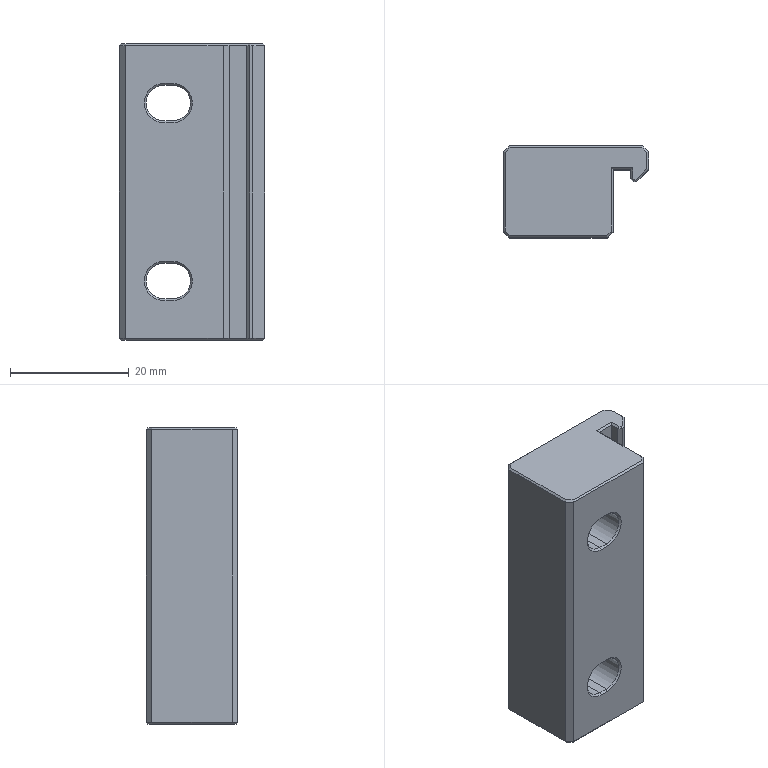Part | SolidWorks | features BaseBody 1 | 1 solid | 86 faces | box 24.5 x 15.5 x 50 mm | volume 13570 mm3 | plane 66 | cone 12 | cylinder 8 | commonest cylinder face diameters 6 x4 11 x4